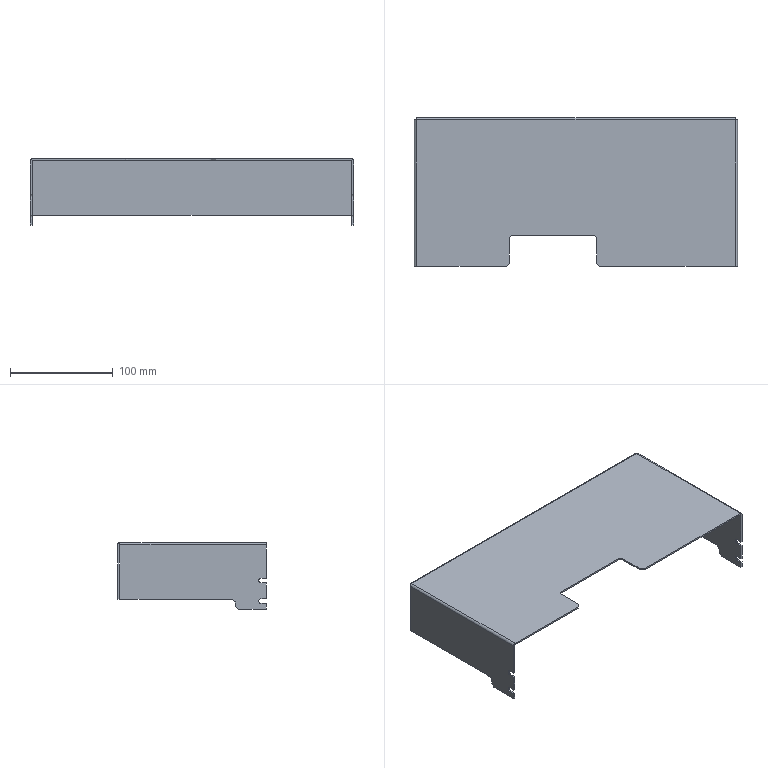Part | NX | features BREP 1 | 1 solid | 62 faces | box 315 x 145 x 65 mm | volume 112650 mm3 | plane 44 | cylinder 14 | spline 4 | commonest cylinder face diameters 4.5 x4 1.473 x3 4.473 x3 6 x2 10 x2